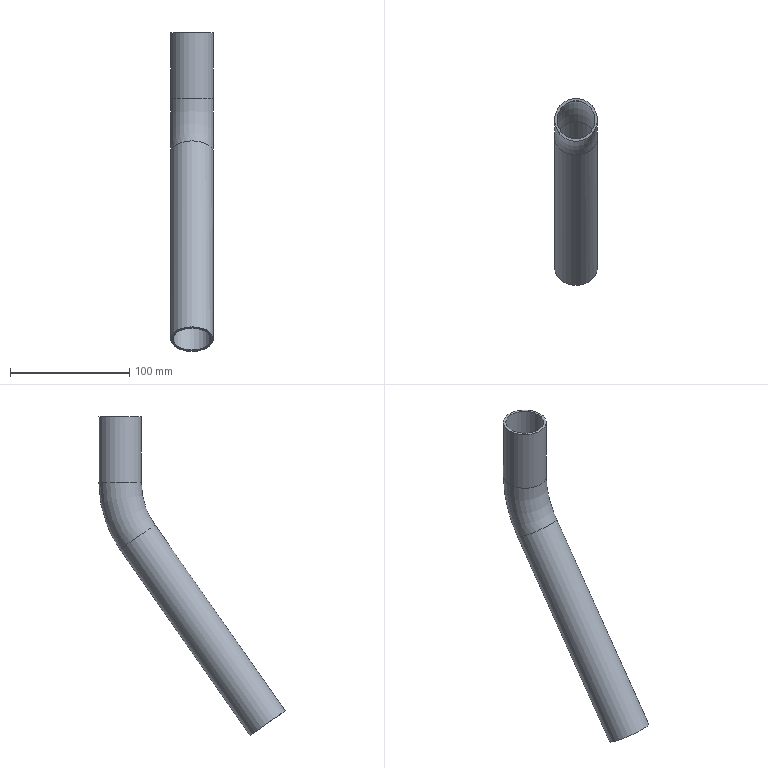Part | STEP file | Q7C1217W | 1 solid | 8 faces | box 35.8 x 156.01 x 266.792 mm | volume 62409 mm3 | cylinder 4 | torus 2 | plane 2 | commonest cylinder face diameters 31.8 x2 35.8 x2
STEP:
#1=CARTESIAN_POINT('',(0.,0.,0.));
#2=DIRECTION('',(0.,0.,1.));
#3=DIRECTION('',(1.,0.,0.));
#4=AXIS2_PLACEMENT_3D('',#1,#2,#3);
#5=CARTESIAN_POINT('',(0.,-29.131,-90.619));
#6=VERTEX_POINT('',#5);
#7=CARTESIAN_POINT('',(17.9,-14.468,-100.886));
#8=VERTEX_POINT('',#7);
#9=CARTESIAN_POINT('',(0.,-14.468,-100.886));
#10=DIRECTION('',(0.,0.5736,0.8192));
#11=DIRECTION('',(0.,-0.8192,0.5736));
#12=AXIS2_PLACEMENT_3D('',#9,#10,#11);
#13=CIRCLE('',#12,17.9);
#14=CARTESIAN_POINT('',(0.,-14.468,-100.886));
#15=DIRECTION('',(0.,-0.5736,-0.8192));
#16=DIRECTION('',(0.,0.8192,-0.5736));
#17=AXIS2_PLACEMENT_3D('',#14,#15,#16);
#18=CYLINDRICAL_SURFACE('',#17,17.9);
#19=CARTESIAN_POINT('',(9.425,0.));
#20=DIRECTION('',(-1.,0.));
#21=VECTOR('',#20,1.);
#22=LINE('',#19,#21);
#23=(GEOMETRIC_REPRESENTATION_CONTEXT(2)PARAMETRIC_REPRESENTATION_CONTEXT()REPRESENTATION_CONTEXT('',''));
#24=DEFINITIONAL_REPRESENTATION('',(#22),#23);
#25=PCURVE('',#18,#24);
#26=CARTESIAN_POINT('',(0.,-80.,-55.));
#27=DIRECTION('',(-1.,0.,0.));
#28=DIRECTION('',(0.,0.,1.));
#29=AXIS2_PLACEMENT_3D('',#26,#27,#28);
#30=TOROIDAL_SURFACE('',#29,80.,17.9);
#31=CARTESIAN_POINT('',(8.465,9.425));
#32=DIRECTION('',(0.,1.));
#33=VECTOR('',#32,1.);
#34=LINE('',#31,#33);
#35=(GEOMETRIC_REPRESENTATION_CONTEXT(2)PARAMETRIC_REPRESENTATION_CONTEXT()REPRESENTATION_CONTEXT('',''));
#36=DEFINITIONAL_REPRESENTATION('',(#34),#35);
#37=PCURVE('',#30,#36);
#38=SURFACE_CURVE('',#13,(#25,#37),.PCURVE_S1.);
#39=EDGE_CURVE('',#6,#8,#38,.T.);
#40=ORIENTED_EDGE('',*,*,#39,.F.);
#41=CARTESIAN_POINT('',(0.,-138.11,-246.258));
#42=VERTEX_POINT('',#41);
#43=CARTESIAN_POINT('',(0.,-29.131,-90.619));
#44=CARTESIAN_POINT('',(0.,-138.11,-246.258));
#45=B_SPLINE_CURVE_WITH_KNOTS('',1,(#43,#44),.UNSPECIFIED.,.F.,.F.,(2,2),(0.,190.),.PIECEWISE_BEZIER_KNOTS.);
#46=CARTESIAN_POINT('',(9.425,0.));
#47=DIRECTION('',(0.,1.));
#48=VECTOR('',#47,1.);
#49=LINE('',#46,#48);
#50=(GEOMETRIC_REPRESENTATION_CONTEXT(2)PARAMETRIC_REPRESENTATION_CONTEXT()REPRESENTATION_CONTEXT('',''));
#51=DEFINITIONAL_REPRESENTATION('',(#49),#50);
#52=PCURVE('',#18,#51);
#53=CARTESIAN_POINT('',(3.142,0.));
#54=DIRECTION('',(0.,1.));
#55=VECTOR('',#54,1.);
#56=LINE('',#53,#55);
#57=(GEOMETRIC_REPRESENTATION_CONTEXT(2)PARAMETRIC_REPRESENTATION_CONTEXT()REPRESENTATION_CONTEXT('',''));
#58=DEFINITIONAL_REPRESENTATION('',(#56),#57);
#59=PCURVE('',#18,#58);
#60=SEAM_CURVE('',#45,(#52,#59),.PCURVE_S1.);
#61=EDGE_CURVE('',#6,#42,#60,.T.);
#62=ORIENTED_EDGE('',*,*,#61,.T.);
#63=CARTESIAN_POINT('',(0.,-123.447,-256.525));
#64=DIRECTION('',(0.,0.5736,0.8192));
#65=DIRECTION('',(0.,-0.8192,0.5736));
#66=AXIS2_PLACEMENT_3D('',#63,#64,#65);
#67=CIRCLE('',#66,17.9);
#68=CARTESIAN_POINT('',(9.425,190.));
#69=DIRECTION('',(-1.,0.));
#70=VECTOR('',#69,1.);
#71=LINE('',#68,#70);
#72=(GEOMETRIC_REPRESENTATION_CONTEXT(2)PARAMETRIC_REPRESENTATION_CONTEXT()REPRESENTATION_CONTEXT('',''));
#73=DEFINITIONAL_REPRESENTATION('',(#71),#72);
#74=PCURVE('',#18,#73);
#75=CARTESIAN_POINT('',(0.,-123.447,-256.525));
#76=DIRECTION('',(0.,0.5736,0.8192));
#77=DIRECTION('',(1.,0.,0.));
#78=AXIS2_PLACEMENT_3D('',#75,#76,#77);
#79=PLANE('',#78);
#80=CARTESIAN_POINT('',(0.,0.));
#81=DIRECTION('',(0.,-1.));
#82=AXIS2_PLACEMENT_2D('',#80,#81);
#83=CIRCLE('',#82,17.9);
#84=(GEOMETRIC_REPRESENTATION_CONTEXT(2)PARAMETRIC_REPRESENTATION_CONTEXT()REPRESENTATION_CONTEXT('',''));
#85=DEFINITIONAL_REPRESENTATION('',(#83),#84);
#86=PCURVE('',#79,#85);
#87=SURFACE_CURVE('',#67,(#74,#86),.PCURVE_S1.);
#88=EDGE_CURVE('',#42,#42,#87,.T.);
#89=ORIENTED_EDGE('',*,*,#88,.T.);
#90=ORIENTED_EDGE('',*,*,#61,.F.);
#91=CARTESIAN_POINT('',(0.,-14.468,-100.886));
#92=DIRECTION('',(0.,0.5736,0.8192));
#93=DIRECTION('',(0.,-0.8192,0.5736));
#94=AXIS2_PLACEMENT_3D('',#91,#92,#93);
#95=CIRCLE('',#94,17.9);
#96=CARTESIAN_POINT('',(9.425,0.));
#97=DIRECTION('',(-1.,0.));
#98=VECTOR('',#97,1.);
#99=LINE('',#96,#98);
#100=(GEOMETRIC_REPRESENTATION_CONTEXT(2)PARAMETRIC_REPRESENTATION_CONTEXT()REPRESENTATION_CONTEXT('',''));
#101=DEFINITIONAL_REPRESENTATION('',(#99),#100);
#102=PCURVE('',#18,#101);
#103=CARTESIAN_POINT('',(8.465,3.142));
#104=DIRECTION('',(0.,1.));
#105=VECTOR('',#104,1.);
#106=LINE('',#103,#105);
#107=(GEOMETRIC_REPRESENTATION_CONTEXT(2)PARAMETRIC_REPRESENTATION_CONTEXT()REPRESENTATION_CONTEXT('',''));
#108=DEFINITIONAL_REPRESENTATION('',(#106),#107);
#109=PCURVE('',#30,#108);
#110=SURFACE_CURVE('',#95,(#102,#109),.PCURVE_S1.);
#111=EDGE_CURVE('',#8,#6,#110,.T.);
#112=ORIENTED_EDGE('',*,*,#111,.F.);
#113=EDGE_LOOP('',(#40,#62,#89,#90,#112));
#114=FACE_BOUND('',#113,.T.);
#115=ADVANCED_FACE('',(#114),#18,.T.);
#116=CARTESIAN_POINT('',(17.9,0.,-55.));
#117=VERTEX_POINT('',#116);
#118=CARTESIAN_POINT('',(0.,0.,-55.));
#119=DIRECTION('',(0.,0.,1.));
#120=DIRECTION('',(1.,0.,0.));
#121=AXIS2_PLACEMENT_3D('',#118,#119,#120);
#122=CIRCLE('',#121,17.9);
#123=CARTESIAN_POINT('',(7.854,4.712));
#124=DIRECTION('',(0.,1.));
#125=VECTOR('',#124,1.);
#126=LINE('',#123,#125);
#127=(GEOMETRIC_REPRESENTATION_CONTEXT(2)PARAMETRIC_REPRESENTATION_CONTEXT()REPRESENTATION_CONTEXT('',''));
#128=DEFINITIONAL_REPRESENTATION('',(#126),#127);
#129=PCURVE('',#30,#128);
#130=CARTESIAN_POINT('',(0.,0.,-55.));
#131=DIRECTION('',(0.,0.,1.));
#132=DIRECTION('',(1.,0.,0.));
#133=AXIS2_PLACEMENT_3D('',#130,#131,#132);
#134=CYLINDRICAL_SURFACE('',#133,17.9);
#135=CARTESIAN_POINT('',(0.,0.));
#136=DIRECTION('',(1.,0.));
#137=VECTOR('',#136,1.);
#138=LINE('',#135,#137);
#139=(GEOMETRIC_REPRESENTATION_CONTEXT(2)PARAMETRIC_REPRESENTATION_CONTEXT()REPRESENTATION_CONTEXT('',''));
#140=DEFINITIONAL_REPRESENTATION('',(#138),#139);
#141=PCURVE('',#134,#140);
#142=SURFACE_CURVE('',#122,(#129,#141),.PCURVE_S1.);
#143=EDGE_CURVE('',#117,#117,#142,.T.);
#144=ORIENTED_EDGE('',*,*,#143,.F.);
#145=CARTESIAN_POINT('',(17.9,0.,-55.));
#146=CARTESIAN_POINT('',(17.9,0.,-63.17));
#147=CARTESIAN_POINT('',(17.9,-1.,-71.31));
#148=CARTESIAN_POINT('',(17.9,-2.988,-79.282));
#149=CARTESIAN_POINT('',(17.9,-5.932,-86.952));
#150=CARTESIAN_POINT('',(17.9,-9.782,-94.193));
#151=CARTESIAN_POINT('',(17.9,-14.468,-100.886));
#152=(BOUNDED_CURVE()B_SPLINE_CURVE(6,(#145,#146,#147,#148,#149,#150,#151),.UNSPECIFIED.,.F.,.F.)B_SPLINE_CURVE_WITH_KNOTS((7,7),(1.571,2.182),.PIECEWISE_BEZIER_KNOTS.)CURVE()GEOMETRIC_REPRESENTATION_ITEM()RATIONAL_B_SPLINE_CURVE((1.005,1.002,0.9997,0.9991,0.9997,1.002,1.005))REPRESENTATION_ITEM(''));
#153=CARTESIAN_POINT('',(6.283,4.712));
#154=DIRECTION('',(1.,0.));
#155=VECTOR('',#154,1.);
#156=LINE('',#153,#155);
#157=(GEOMETRIC_REPRESENTATION_CONTEXT(2)PARAMETRIC_REPRESENTATION_CONTEXT()REPRESENTATION_CONTEXT('',''));
#158=DEFINITIONAL_REPRESENTATION('',(#156),#157);
#159=PCURVE('',#30,#158);
#160=CARTESIAN_POINT('',(6.283,10.996));
#161=DIRECTION('',(1.,0.));
#162=VECTOR('',#161,1.);
#163=LINE('',#160,#162);
#164=(GEOMETRIC_REPRESENTATION_CONTEXT(2)PARAMETRIC_REPRESENTATION_CONTEXT()REPRESENTATION_CONTEXT('',''));
#165=DEFINITIONAL_REPRESENTATION('',(#163),#164);
#166=PCURVE('',#30,#165);
#167=SEAM_CURVE('',#152,(#159,#166),.PCURVE_S1.);
#168=EDGE_CURVE('',#117,#8,#167,.T.);
#169=ORIENTED_EDGE('',*,*,#168,.T.);
#170=ORIENTED_EDGE('',*,*,#111,.T.);
#171=ORIENTED_EDGE('',*,*,#39,.T.);
#172=ORIENTED_EDGE('',*,*,#168,.F.);
#173=EDGE_LOOP('',(#144,#169,#170,#171,#172));
#174=FACE_BOUND('',#173,.T.);
#175=ADVANCED_FACE('',(#174),#30,.T.);
#176=ORIENTED_EDGE('',*,*,#143,.T.);
#177=CARTESIAN_POINT('',(17.9,0.,0.));
#178=VERTEX_POINT('',#177);
#179=CARTESIAN_POINT('',(17.9,0.,-55.));
#180=CARTESIAN_POINT('',(17.9,0.,0.));
#181=B_SPLINE_CURVE_WITH_KNOTS('',1,(#179,#180),.UNSPECIFIED.,.F.,.F.,(2,2),(0.,55.),.PIECEWISE_BEZIER_KNOTS.);
#182=CARTESIAN_POINT('',(6.283,0.));
#183=DIRECTION('',(0.,1.));
#184=VECTOR('',#183,1.);
#185=LINE('',#182,#184);
#186=(GEOMETRIC_REPRESENTATION_CONTEXT(2)PARAMETRIC_REPRESENTATION_CONTEXT()REPRESENTATION_CONTEXT('',''));
#187=DEFINITIONAL_REPRESENTATION('',(#185),#186);
#188=PCURVE('',#134,#187);
#189=CARTESIAN_POINT('',(0.,0.));
#190=DIRECTION('',(0.,1.));
#191=VECTOR('',#190,1.);
#192=LINE('',#189,#191);
#193=(GEOMETRIC_REPRESENTATION_CONTEXT(2)PARAMETRIC_REPRESENTATION_CONTEXT()REPRESENTATION_CONTEXT('',''));
#194=DEFINITIONAL_REPRESENTATION('',(#192),#193);
#195=PCURVE('',#134,#194);
#196=SEAM_CURVE('',#181,(#188,#195),.PCURVE_S1.);
#197=EDGE_CURVE('',#117,#178,#196,.T.);
#198=ORIENTED_EDGE('',*,*,#197,.T.);
#199=CARTESIAN_POINT('',(0.,0.,0.));
#200=DIRECTION('',(0.,0.,1.));
#201=DIRECTION('',(1.,0.,0.));
#202=AXIS2_PLACEMENT_3D('',#199,#200,#201);
#203=CIRCLE('',#202,17.9);
#204=CARTESIAN_POINT('',(0.,55.));
#205=DIRECTION('',(1.,0.));
#206=VECTOR('',#205,1.);
#207=LINE('',#204,#206);
#208=(GEOMETRIC_REPRESENTATION_CONTEXT(2)PARAMETRIC_REPRESENTATION_CONTEXT()REPRESENTATION_CONTEXT('',''));
#209=DEFINITIONAL_REPRESENTATION('',(#207),#208);
#210=PCURVE('',#134,#209);
#211=CARTESIAN_POINT('',(0.,0.,0.));
#212=DIRECTION('',(0.,0.,1.));
#213=DIRECTION('',(1.,0.,0.));
#214=AXIS2_PLACEMENT_3D('',#211,#212,#213);
#215=PLANE('',#214);
#216=CARTESIAN_POINT('',(0.,0.));
#217=DIRECTION('',(1.,0.));
#218=AXIS2_PLACEMENT_2D('',#216,#217);
#219=CIRCLE('',#218,17.9);
#220=(GEOMETRIC_REPRESENTATION_CONTEXT(2)PARAMETRIC_REPRESENTATION_CONTEXT()REPRESENTATION_CONTEXT('',''));
#221=DEFINITIONAL_REPRESENTATION('',(#219),#220);
#222=PCURVE('',#215,#221);
#223=SURFACE_CURVE('',#203,(#210,#222),.PCURVE_S1.);
#224=EDGE_CURVE('',#178,#178,#223,.T.);
#225=ORIENTED_EDGE('',*,*,#224,.F.);
#226=ORIENTED_EDGE('',*,*,#197,.F.);
#227=EDGE_LOOP('',(#176,#198,#225,#226));
#228=FACE_BOUND('',#227,.T.);
#229=ADVANCED_FACE('',(#228),#134,.T.);
#230=CARTESIAN_POINT('',(15.9,-123.447,-256.525));
#231=VERTEX_POINT('',#230);
#232=CARTESIAN_POINT('',(0.,-123.447,-256.525));
#233=DIRECTION('',(0.,0.5736,0.8192));
#234=DIRECTION('',(1.,0.,0.));
#235=AXIS2_PLACEMENT_3D('',#232,#233,#234);
#236=CIRCLE('',#235,15.9);
#237=CARTESIAN_POINT('',(0.,0.));
#238=DIRECTION('',(1.,0.));
#239=AXIS2_PLACEMENT_2D('',#237,#238);
#240=CIRCLE('',#239,15.9);
#241=(GEOMETRIC_REPRESENTATION_CONTEXT(2)PARAMETRIC_REPRESENTATION_CONTEXT()REPRESENTATION_CONTEXT('',''));
#242=DEFINITIONAL_REPRESENTATION('',(#240),#241);
#243=PCURVE('',#79,#242);
#244=CARTESIAN_POINT('',(0.,-14.468,-100.886));
#245=DIRECTION('',(0.,-0.5736,-0.8192));
#246=DIRECTION('',(0.,0.8192,-0.5736));
#247=AXIS2_PLACEMENT_3D('',#244,#245,#246);
#248=CYLINDRICAL_SURFACE('',#247,15.9);
#249=CARTESIAN_POINT('',(7.854,190.));
#250=DIRECTION('',(-1.,0.));
#251=VECTOR('',#250,1.);
#252=LINE('',#249,#251);
#253=(GEOMETRIC_REPRESENTATION_CONTEXT(2)PARAMETRIC_REPRESENTATION_CONTEXT()REPRESENTATION_CONTEXT('',''));
#254=DEFINITIONAL_REPRESENTATION('',(#252),#253);
#255=PCURVE('',#248,#254);
#256=SURFACE_CURVE('',#236,(#243,#255),.PCURVE_S1.);
#257=EDGE_CURVE('',#231,#231,#256,.T.);
#258=ORIENTED_EDGE('',*,*,#257,.T.);
#259=EDGE_LOOP('',(#258));
#260=FACE_BOUND('',#259,.T.);
#261=ORIENTED_EDGE('',*,*,#88,.F.);
#262=EDGE_LOOP('',(#261));
#263=FACE_BOUND('',#262,.T.);
#264=ADVANCED_FACE('',(#260,#263),#79,.F.);
#265=CARTESIAN_POINT('',(15.9,0.,0.));
#266=VERTEX_POINT('',#265);
#267=CARTESIAN_POINT('',(0.,0.,0.));
#268=DIRECTION('',(0.,0.,1.));
#269=DIRECTION('',(1.,0.,0.));
#270=AXIS2_PLACEMENT_3D('',#267,#268,#269);
#271=CIRCLE('',#270,15.9);
#272=CARTESIAN_POINT('',(0.,0.));
#273=DIRECTION('',(1.,0.));
#274=AXIS2_PLACEMENT_2D('',#272,#273);
#275=CIRCLE('',#274,15.9);
#276=(GEOMETRIC_REPRESENTATION_CONTEXT(2)PARAMETRIC_REPRESENTATION_CONTEXT()REPRESENTATION_CONTEXT('',''));
#277=DEFINITIONAL_REPRESENTATION('',(#275),#276);
#278=PCURVE('',#215,#277);
#279=CARTESIAN_POINT('',(0.,0.,-55.));
#280=DIRECTION('',(0.,0.,1.));
#281=DIRECTION('',(1.,0.,0.));
#282=AXIS2_PLACEMENT_3D('',#279,#280,#281);
#283=CYLINDRICAL_SURFACE('',#282,15.9);
#284=CARTESIAN_POINT('',(0.,55.));
#285=DIRECTION('',(1.,0.));
#286=VECTOR('',#285,1.);
#287=LINE('',#284,#286);
#288=(GEOMETRIC_REPRESENTATION_CONTEXT(2)PARAMETRIC_REPRESENTATION_CONTEXT()REPRESENTATION_CONTEXT('',''));
#289=DEFINITIONAL_REPRESENTATION('',(#287),#288);
#290=PCURVE('',#283,#289);
#291=SURFACE_CURVE('',#271,(#278,#290),.PCURVE_S1.);
#292=EDGE_CURVE('',#266,#266,#291,.T.);
#293=ORIENTED_EDGE('',*,*,#292,.F.);
#294=EDGE_LOOP('',(#293));
#295=FACE_BOUND('',#294,.T.);
#296=ORIENTED_EDGE('',*,*,#224,.T.);
#297=EDGE_LOOP('',(#296));
#298=FACE_BOUND('',#297,.T.);
#299=ADVANCED_FACE('',(#295,#298),#215,.T.);
#300=CARTESIAN_POINT('',(15.9,-14.468,-100.886));
#301=VERTEX_POINT('',#300);
#302=CARTESIAN_POINT('',(0.,-14.468,-100.886));
#303=DIRECTION('',(0.,0.5736,0.8192));
#304=DIRECTION('',(1.,0.,0.));
#305=AXIS2_PLACEMENT_3D('',#302,#303,#304);
#306=CIRCLE('',#305,15.9);
#307=CARTESIAN_POINT('',(7.854,0.));
#308=DIRECTION('',(-1.,0.));
#309=VECTOR('',#308,1.);
#310=LINE('',#307,#309);
#311=(GEOMETRIC_REPRESENTATION_CONTEXT(2)PARAMETRIC_REPRESENTATION_CONTEXT()REPRESENTATION_CONTEXT('',''));
#312=DEFINITIONAL_REPRESENTATION('',(#310),#311);
#313=PCURVE('',#248,#312);
#314=CARTESIAN_POINT('',(0.,-80.,-55.));
#315=DIRECTION('',(-1.,0.,0.));
#316=DIRECTION('',(0.,0.,1.));
#317=AXIS2_PLACEMENT_3D('',#314,#315,#316);
#318=TOROIDAL_SURFACE('',#317,80.,15.9);
#319=CARTESIAN_POINT('',(8.465,4.712));
#320=DIRECTION('',(0.,1.));
#321=VECTOR('',#320,1.);
#322=LINE('',#319,#321);
#323=(GEOMETRIC_REPRESENTATION_CONTEXT(2)PARAMETRIC_REPRESENTATION_CONTEXT()REPRESENTATION_CONTEXT('',''));
#324=DEFINITIONAL_REPRESENTATION('',(#322),#323);
#325=PCURVE('',#318,#324);
#326=SURFACE_CURVE('',#306,(#313,#325),.PCURVE_S1.);
#327=EDGE_CURVE('',#301,#301,#326,.T.);
#328=ORIENTED_EDGE('',*,*,#327,.F.);
#329=CARTESIAN_POINT('',(15.9,-14.468,-100.886));
#330=CARTESIAN_POINT('',(15.9,-123.447,-256.525));
#331=B_SPLINE_CURVE_WITH_KNOTS('',1,(#329,#330),.UNSPECIFIED.,.F.,.F.,(2,2),(0.,190.),.PIECEWISE_BEZIER_KNOTS.);
#332=CARTESIAN_POINT('',(7.854,0.));
#333=DIRECTION('',(0.,1.));
#334=VECTOR('',#333,1.);
#335=LINE('',#332,#334);
#336=(GEOMETRIC_REPRESENTATION_CONTEXT(2)PARAMETRIC_REPRESENTATION_CONTEXT()REPRESENTATION_CONTEXT('',''));
#337=DEFINITIONAL_REPRESENTATION('',(#335),#336);
#338=PCURVE('',#248,#337);
#339=CARTESIAN_POINT('',(1.571,0.));
#340=DIRECTION('',(0.,1.));
#341=VECTOR('',#340,1.);
#342=LINE('',#339,#341);
#343=(GEOMETRIC_REPRESENTATION_CONTEXT(2)PARAMETRIC_REPRESENTATION_CONTEXT()REPRESENTATION_CONTEXT('',''));
#344=DEFINITIONAL_REPRESENTATION('',(#342),#343);
#345=PCURVE('',#248,#344);
#346=SEAM_CURVE('',#331,(#338,#345),.PCURVE_S1.);
#347=EDGE_CURVE('',#301,#231,#346,.T.);
#348=ORIENTED_EDGE('',*,*,#347,.T.);
#349=ORIENTED_EDGE('',*,*,#257,.T.);
#350=ORIENTED_EDGE('',*,*,#347,.F.);
#351=EDGE_LOOP('',(#328,#348,#349,#350));
#352=FACE_BOUND('',#351,.F.);
#353=ADVANCED_FACE('',(#352),#248,.F.);
#354=CARTESIAN_POINT('',(15.9,0.,-55.));
#355=VERTEX_POINT('',#354);
#356=CARTESIAN_POINT('',(0.,0.,-55.));
#357=DIRECTION('',(0.,0.,1.));
#358=DIRECTION('',(1.,0.,0.));
#359=AXIS2_PLACEMENT_3D('',#356,#357,#358);
#360=CIRCLE('',#359,15.9);
#361=CARTESIAN_POINT('',(7.854,4.712));
#362=DIRECTION('',(0.,1.));
#363=VECTOR('',#362,1.);
#364=LINE('',#361,#363);
#365=(GEOMETRIC_REPRESENTATION_CONTEXT(2)PARAMETRIC_REPRESENTATION_CONTEXT()REPRESENTATION_CONTEXT('',''));
#366=DEFINITIONAL_REPRESENTATION('',(#364),#365);
#367=PCURVE('',#318,#366);
#368=CARTESIAN_POINT('',(0.,0.));
#369=DIRECTION('',(1.,0.));
#370=VECTOR('',#369,1.);
#371=LINE('',#368,#370);
#372=(GEOMETRIC_REPRESENTATION_CONTEXT(2)PARAMETRIC_REPRESENTATION_CONTEXT()REPRESENTATION_CONTEXT('',''));
#373=DEFINITIONAL_REPRESENTATION('',(#371),#372);
#374=PCURVE('',#283,#373);
#375=SURFACE_CURVE('',#360,(#367,#374),.PCURVE_S1.);
#376=EDGE_CURVE('',#355,#355,#375,.T.);
#377=ORIENTED_EDGE('',*,*,#376,.F.);
#378=CARTESIAN_POINT('',(15.9,0.,-55.));
#379=CARTESIAN_POINT('',(15.9,0.,-63.17));
#380=CARTESIAN_POINT('',(15.9,-1.,-71.31));
#381=CARTESIAN_POINT('',(15.9,-2.988,-79.282));
#382=CARTESIAN_POINT('',(15.9,-5.932,-86.952));
#383=CARTESIAN_POINT('',(15.9,-9.782,-94.193));
#384=CARTESIAN_POINT('',(15.9,-14.468,-100.886));
#385=(BOUNDED_CURVE()B_SPLINE_CURVE(6,(#378,#379,#380,#381,#382,#383,#384),.UNSPECIFIED.,.F.,.F.)B_SPLINE_CURVE_WITH_KNOTS((7,7),(1.571,2.182),.PIECEWISE_BEZIER_KNOTS.)CURVE()GEOMETRIC_REPRESENTATION_ITEM()RATIONAL_B_SPLINE_CURVE((1.005,1.002,0.9997,0.9991,0.9997,1.002,1.005))REPRESENTATION_ITEM(''));
#386=CARTESIAN_POINT('',(6.283,4.712));
#387=DIRECTION('',(1.,0.));
#388=VECTOR('',#387,1.);
#389=LINE('',#386,#388);
#390=(GEOMETRIC_REPRESENTATION_CONTEXT(2)PARAMETRIC_REPRESENTATION_CONTEXT()REPRESENTATION_CONTEXT('',''));
#391=DEFINITIONAL_REPRESENTATION('',(#389),#390);
#392=PCURVE('',#318,#391);
#393=CARTESIAN_POINT('',(6.283,10.996));
#394=DIRECTION('',(1.,0.));
#395=VECTOR('',#394,1.);
#396=LINE('',#393,#395);
#397=(GEOMETRIC_REPRESENTATION_CONTEXT(2)PARAMETRIC_REPRESENTATION_CONTEXT()REPRESENTATION_CONTEXT('',''));
#398=DEFINITIONAL_REPRESENTATION('',(#396),#397);
#399=PCURVE('',#318,#398);
#400=SEAM_CURVE('',#385,(#392,#399),.PCURVE_S1.);
#401=EDGE_CURVE('',#355,#301,#400,.T.);
#402=ORIENTED_EDGE('',*,*,#401,.T.);
#403=ORIENTED_EDGE('',*,*,#327,.T.);
#404=ORIENTED_EDGE('',*,*,#401,.F.);
#405=EDGE_LOOP('',(#377,#402,#403,#404));
#406=FACE_BOUND('',#405,.F.);
#407=ADVANCED_FACE('',(#406),#318,.F.);
#408=ORIENTED_EDGE('',*,*,#376,.T.);
#409=CARTESIAN_POINT('',(15.9,0.,-55.));
#410=CARTESIAN_POINT('',(15.9,0.,0.));
#411=B_SPLINE_CURVE_WITH_KNOTS('',1,(#409,#410),.UNSPECIFIED.,.F.,.F.,(2,2),(0.,55.),.PIECEWISE_BEZIER_KNOTS.);
#412=CARTESIAN_POINT('',(6.283,0.));
#413=DIRECTION('',(0.,1.));
#414=VECTOR('',#413,1.);
#415=LINE('',#412,#414);
#416=(GEOMETRIC_REPRESENTATION_CONTEXT(2)PARAMETRIC_REPRESENTATION_CONTEXT()REPRESENTATION_CONTEXT('',''));
#417=DEFINITIONAL_REPRESENTATION('',(#415),#416);
#418=PCURVE('',#283,#417);
#419=CARTESIAN_POINT('',(0.,0.));
#420=DIRECTION('',(0.,1.));
#421=VECTOR('',#420,1.);
#422=LINE('',#419,#421);
#423=(GEOMETRIC_REPRESENTATION_CONTEXT(2)PARAMETRIC_REPRESENTATION_CONTEXT()REPRESENTATION_CONTEXT('',''));
#424=DEFINITIONAL_REPRESENTATION('',(#422),#423);
#425=PCURVE('',#283,#424);
#426=SEAM_CURVE('',#411,(#418,#425),.PCURVE_S1.);
#427=EDGE_CURVE('',#355,#266,#426,.T.);
#428=ORIENTED_EDGE('',*,*,#427,.T.);
#429=ORIENTED_EDGE('',*,*,#292,.F.);
#430=ORIENTED_EDGE('',*,*,#427,.F.);
#431=EDGE_LOOP('',(#408,#428,#429,#430));
#432=FACE_BOUND('',#431,.F.);
#433=ADVANCED_FACE('',(#432),#283,.F.);
#434=CLOSED_SHELL('',(#115,#175,#229,#264,#299,#353,#407,#433));
#435=MANIFOLD_SOLID_BREP('',#434);
#436=(LENGTH_UNIT()NAMED_UNIT(*)SI_UNIT(.MILLI.,.METRE.));
#437=UNCERTAINTY_MEASURE_WITH_UNIT(LENGTH_MEASURE(0.00001),#436,'','');
#438=(NAMED_UNIT(*)PLANE_ANGLE_UNIT()SI_UNIT($,.RADIAN.));
#439=(NAMED_UNIT(*)SI_UNIT($,.STERADIAN.)SOLID_ANGLE_UNIT());
#440=(GEOMETRIC_REPRESENTATION_CONTEXT(3)GLOBAL_UNCERTAINTY_ASSIGNED_CONTEXT((#437))GLOBAL_UNIT_ASSIGNED_CONTEXT((#436,#438,#439))REPRESENTATION_CONTEXT('',''));
#441=ADVANCED_BREP_SHAPE_REPRESENTATION('',(#4,#435),#440);